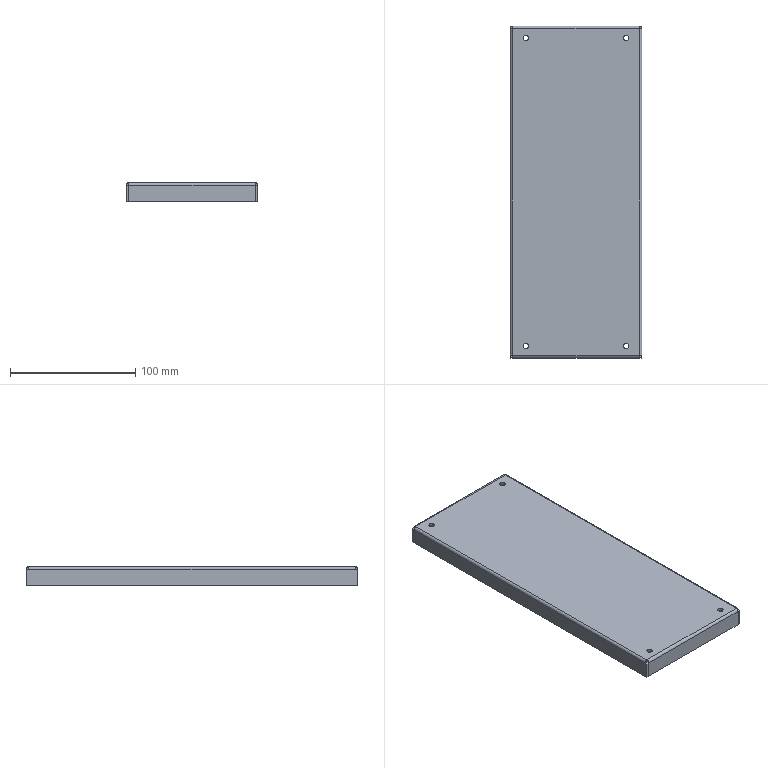Part | SolidWorks | features BaseBody 1 | 1 solid | 46 faces | box 105 x 265 x 15 mm | volume 73841 mm3 | plane 30 | cylinder 16 | commonest cylinder face diameters 4.2 x12 0.2 x4
STEP:
#1=CARTESIAN_POINT('',(37.9,-123.,-2.));
#2=VERTEX_POINT('',#1);
#3=CARTESIAN_POINT('',(42.1,-123.,-2.));
#4=VERTEX_POINT('',#3);
#5=CARTESIAN_POINT('',(40.,-123.,-2.));
#6=DIRECTION('',(0.,0.,1.));
#7=DIRECTION('',(1.,0.,0.));
#8=AXIS2_PLACEMENT_3D('',#5,#6,#7);
#9=CIRCLE('',#8,2.1);
#10=EDGE_CURVE('',#2,#4,#9,.T.);
#11=ORIENTED_EDGE('',*,*,#10,.F.);
#12=CARTESIAN_POINT('',(37.9,-123.,0.));
#13=VERTEX_POINT('',#12);
#14=CARTESIAN_POINT('',(37.9,-123.,0.));
#15=DIRECTION('',(0.,0.,1.));
#16=VECTOR('',#15,1000.);
#17=LINE('',#14,#16);
#18=EDGE_CURVE('',#2,#13,#17,.T.);
#19=ORIENTED_EDGE('',*,*,#18,.T.);
#20=CARTESIAN_POINT('',(42.1,-123.,0.));
#21=VERTEX_POINT('',#20);
#22=CARTESIAN_POINT('',(40.,-123.,0.));
#23=DIRECTION('',(0.,0.,-1.));
#24=DIRECTION('',(1.,0.,0.));
#25=AXIS2_PLACEMENT_3D('',#22,#23,#24);
#26=CIRCLE('',#25,2.1);
#27=EDGE_CURVE('',#21,#13,#26,.T.);
#28=ORIENTED_EDGE('',*,*,#27,.F.);
#29=CARTESIAN_POINT('',(42.1,-123.,0.));
#30=DIRECTION('',(0.,0.,1.));
#31=VECTOR('',#30,1000.);
#32=LINE('',#29,#31);
#33=EDGE_CURVE('',#4,#21,#32,.T.);
#34=ORIENTED_EDGE('',*,*,#33,.F.);
#35=EDGE_LOOP('',(#11,#19,#28,#34));
#36=FACE_OUTER_BOUND('',#35,.T.);
#37=CARTESIAN_POINT('',(40.,-123.,0.));
#38=DIRECTION('',(0.,0.,1.));
#39=DIRECTION('',(1.,0.,0.));
#40=AXIS2_PLACEMENT_3D('',#37,#38,#39);
#41=CYLINDRICAL_SURFACE('',#40,2.1);
#42=ADVANCED_FACE('',(#36),#41,.F.);
#43=CARTESIAN_POINT('',(-42.1,-123.,-2.));
#44=VERTEX_POINT('',#43);
#45=CARTESIAN_POINT('',(-37.9,-123.,-2.));
#46=VERTEX_POINT('',#45);
#47=CARTESIAN_POINT('',(-40.,-123.,-2.));
#48=DIRECTION('',(0.,0.,1.));
#49=DIRECTION('',(1.,0.,0.));
#50=AXIS2_PLACEMENT_3D('',#47,#48,#49);
#51=CIRCLE('',#50,2.1);
#52=EDGE_CURVE('',#44,#46,#51,.T.);
#53=ORIENTED_EDGE('',*,*,#52,.F.);
#54=CARTESIAN_POINT('',(-42.1,-123.,0.));
#55=VERTEX_POINT('',#54);
#56=CARTESIAN_POINT('',(-42.1,-123.,0.));
#57=DIRECTION('',(0.,0.,1.));
#58=VECTOR('',#57,1000.);
#59=LINE('',#56,#58);
#60=EDGE_CURVE('',#44,#55,#59,.T.);
#61=ORIENTED_EDGE('',*,*,#60,.T.);
#62=CARTESIAN_POINT('',(-37.9,-123.,0.));
#63=VERTEX_POINT('',#62);
#64=CARTESIAN_POINT('',(-40.,-123.,0.));
#65=DIRECTION('',(0.,0.,-1.));
#66=DIRECTION('',(1.,0.,0.));
#67=AXIS2_PLACEMENT_3D('',#64,#65,#66);
#68=CIRCLE('',#67,2.1);
#69=EDGE_CURVE('',#63,#55,#68,.T.);
#70=ORIENTED_EDGE('',*,*,#69,.F.);
#71=CARTESIAN_POINT('',(-37.9,-123.,0.));
#72=DIRECTION('',(0.,0.,1.));
#73=VECTOR('',#72,1000.);
#74=LINE('',#71,#73);
#75=EDGE_CURVE('',#46,#63,#74,.T.);
#76=ORIENTED_EDGE('',*,*,#75,.F.);
#77=EDGE_LOOP('',(#53,#61,#70,#76));
#78=FACE_OUTER_BOUND('',#77,.T.);
#79=CARTESIAN_POINT('',(-40.,-123.,0.));
#80=DIRECTION('',(0.,0.,1.));
#81=DIRECTION('',(1.,0.,0.));
#82=AXIS2_PLACEMENT_3D('',#79,#80,#81);
#83=CYLINDRICAL_SURFACE('',#82,2.1);
#84=ADVANCED_FACE('',(#78),#83,.F.);
#85=CARTESIAN_POINT('',(-42.1,123.,-2.));
#86=VERTEX_POINT('',#85);
#87=CARTESIAN_POINT('',(-37.9,123.,-2.));
#88=VERTEX_POINT('',#87);
#89=CARTESIAN_POINT('',(-40.,123.,-2.));
#90=DIRECTION('',(0.,0.,1.));
#91=DIRECTION('',(1.,0.,0.));
#92=AXIS2_PLACEMENT_3D('',#89,#90,#91);
#93=CIRCLE('',#92,2.1);
#94=EDGE_CURVE('',#86,#88,#93,.T.);
#95=ORIENTED_EDGE('',*,*,#94,.F.);
#96=CARTESIAN_POINT('',(-42.1,123.,0.));
#97=VERTEX_POINT('',#96);
#98=CARTESIAN_POINT('',(-42.1,123.,0.));
#99=DIRECTION('',(0.,0.,1.));
#100=VECTOR('',#99,1000.);
#101=LINE('',#98,#100);
#102=EDGE_CURVE('',#86,#97,#101,.T.);
#103=ORIENTED_EDGE('',*,*,#102,.T.);
#104=CARTESIAN_POINT('',(-37.9,123.,0.));
#105=VERTEX_POINT('',#104);
#106=CARTESIAN_POINT('',(-40.,123.,0.));
#107=DIRECTION('',(0.,0.,-1.));
#108=DIRECTION('',(1.,0.,0.));
#109=AXIS2_PLACEMENT_3D('',#106,#107,#108);
#110=CIRCLE('',#109,2.1);
#111=EDGE_CURVE('',#105,#97,#110,.T.);
#112=ORIENTED_EDGE('',*,*,#111,.F.);
#113=CARTESIAN_POINT('',(-37.9,123.,0.));
#114=DIRECTION('',(0.,0.,1.));
#115=VECTOR('',#114,1000.);
#116=LINE('',#113,#115);
#117=EDGE_CURVE('',#88,#105,#116,.T.);
#118=ORIENTED_EDGE('',*,*,#117,.F.);
#119=EDGE_LOOP('',(#95,#103,#112,#118));
#120=FACE_OUTER_BOUND('',#119,.T.);
#121=CARTESIAN_POINT('',(-40.,123.,0.));
#122=DIRECTION('',(0.,0.,1.));
#123=DIRECTION('',(1.,0.,0.));
#124=AXIS2_PLACEMENT_3D('',#121,#122,#123);
#125=CYLINDRICAL_SURFACE('',#124,2.1);
#126=ADVANCED_FACE('',(#120),#125,.F.);
#127=CARTESIAN_POINT('',(37.9,123.,-2.));
#128=VERTEX_POINT('',#127);
#129=CARTESIAN_POINT('',(42.1,123.,-2.));
#130=VERTEX_POINT('',#129);
#131=CARTESIAN_POINT('',(40.,123.,-2.));
#132=DIRECTION('',(0.,0.,1.));
#133=DIRECTION('',(1.,0.,0.));
#134=AXIS2_PLACEMENT_3D('',#131,#132,#133);
#135=CIRCLE('',#134,2.1);
#136=EDGE_CURVE('',#128,#130,#135,.T.);
#137=ORIENTED_EDGE('',*,*,#136,.F.);
#138=CARTESIAN_POINT('',(37.9,123.,0.));
#139=VERTEX_POINT('',#138);
#140=CARTESIAN_POINT('',(37.9,123.,0.));
#141=DIRECTION('',(0.,0.,1.));
#142=VECTOR('',#141,1000.);
#143=LINE('',#140,#142);
#144=EDGE_CURVE('',#128,#139,#143,.T.);
#145=ORIENTED_EDGE('',*,*,#144,.T.);
#146=CARTESIAN_POINT('',(42.1,123.,0.));
#147=VERTEX_POINT('',#146);
#148=CARTESIAN_POINT('',(40.,123.,0.));
#149=DIRECTION('',(0.,0.,-1.));
#150=DIRECTION('',(1.,0.,0.));
#151=AXIS2_PLACEMENT_3D('',#148,#149,#150);
#152=CIRCLE('',#151,2.1);
#153=EDGE_CURVE('',#147,#139,#152,.T.);
#154=ORIENTED_EDGE('',*,*,#153,.F.);
#155=CARTESIAN_POINT('',(42.1,123.,0.));
#156=DIRECTION('',(0.,0.,1.));
#157=VECTOR('',#156,1000.);
#158=LINE('',#155,#157);
#159=EDGE_CURVE('',#130,#147,#158,.T.);
#160=ORIENTED_EDGE('',*,*,#159,.F.);
#161=EDGE_LOOP('',(#137,#145,#154,#160));
#162=FACE_OUTER_BOUND('',#161,.T.);
#163=CARTESIAN_POINT('',(40.,123.,0.));
#164=DIRECTION('',(0.,0.,1.));
#165=DIRECTION('',(1.,0.,0.));
#166=AXIS2_PLACEMENT_3D('',#163,#164,#165);
#167=CYLINDRICAL_SURFACE('',#166,2.1);
#168=ADVANCED_FACE('',(#162),#167,.F.);
#169=ORIENTED_EDGE('',*,*,#27,.T.);
#170=CARTESIAN_POINT('',(40.,-123.,0.));
#171=DIRECTION('',(0.,0.,-1.));
#172=DIRECTION('',(1.,0.,0.));
#173=AXIS2_PLACEMENT_3D('',#170,#171,#172);
#174=CIRCLE('',#173,2.1);
#175=EDGE_CURVE('',#13,#21,#174,.T.);
#176=ORIENTED_EDGE('',*,*,#175,.T.);
#177=EDGE_LOOP('',(#169,#176));
#178=FACE_BOUND('',#177,.T.);
#179=ORIENTED_EDGE('',*,*,#69,.T.);
#180=CARTESIAN_POINT('',(-40.,-123.,0.));
#181=DIRECTION('',(0.,0.,-1.));
#182=DIRECTION('',(1.,0.,0.));
#183=AXIS2_PLACEMENT_3D('',#180,#181,#182);
#184=CIRCLE('',#183,2.1);
#185=EDGE_CURVE('',#55,#63,#184,.T.);
#186=ORIENTED_EDGE('',*,*,#185,.T.);
#187=EDGE_LOOP('',(#179,#186));
#188=FACE_BOUND('',#187,.T.);
#189=CARTESIAN_POINT('',(50.4,-130.4,0.));
#190=VERTEX_POINT('',#189);
#191=CARTESIAN_POINT('',(50.4,130.4,0.));
#192=VERTEX_POINT('',#191);
#193=CARTESIAN_POINT('',(50.4,0.,0.));
#194=DIRECTION('',(0.,1.,0.));
#195=VECTOR('',#194,1000.);
#196=LINE('',#193,#195);
#197=EDGE_CURVE('',#190,#192,#196,.T.);
#198=ORIENTED_EDGE('',*,*,#197,.T.);
#199=CARTESIAN_POINT('',(-50.4,130.4,0.));
#200=VERTEX_POINT('',#199);
#201=CARTESIAN_POINT('',(0.,130.4,0.));
#202=DIRECTION('',(-1.,0.,0.));
#203=VECTOR('',#202,1000.);
#204=LINE('',#201,#203);
#205=EDGE_CURVE('',#192,#200,#204,.T.);
#206=ORIENTED_EDGE('',*,*,#205,.T.);
#207=CARTESIAN_POINT('',(-50.4,-130.4,0.));
#208=VERTEX_POINT('',#207);
#209=CARTESIAN_POINT('',(-50.4,0.,0.));
#210=DIRECTION('',(0.,-1.,0.));
#211=VECTOR('',#210,1000.);
#212=LINE('',#209,#211);
#213=EDGE_CURVE('',#200,#208,#212,.T.);
#214=ORIENTED_EDGE('',*,*,#213,.T.);
#215=CARTESIAN_POINT('',(0.,-130.4,0.));
#216=DIRECTION('',(1.,0.,0.));
#217=VECTOR('',#216,1000.);
#218=LINE('',#215,#217);
#219=EDGE_CURVE('',#208,#190,#218,.T.);
#220=ORIENTED_EDGE('',*,*,#219,.T.);
#221=EDGE_LOOP('',(#198,#206,#214,#220));
#222=FACE_OUTER_BOUND('',#221,.T.);
#223=ORIENTED_EDGE('',*,*,#111,.T.);
#224=CARTESIAN_POINT('',(-40.,123.,0.));
#225=DIRECTION('',(0.,0.,-1.));
#226=DIRECTION('',(1.,0.,0.));
#227=AXIS2_PLACEMENT_3D('',#224,#225,#226);
#228=CIRCLE('',#227,2.1);
#229=EDGE_CURVE('',#97,#105,#228,.T.);
#230=ORIENTED_EDGE('',*,*,#229,.T.);
#231=EDGE_LOOP('',(#223,#230));
#232=FACE_BOUND('',#231,.T.);
#233=ORIENTED_EDGE('',*,*,#153,.T.);
#234=CARTESIAN_POINT('',(40.,123.,0.));
#235=DIRECTION('',(0.,0.,-1.));
#236=DIRECTION('',(1.,0.,0.));
#237=AXIS2_PLACEMENT_3D('',#234,#235,#236);
#238=CIRCLE('',#237,2.1);
#239=EDGE_CURVE('',#139,#147,#238,.T.);
#240=ORIENTED_EDGE('',*,*,#239,.T.);
#241=EDGE_LOOP('',(#233,#240));
#242=FACE_BOUND('',#241,.T.);
#243=CARTESIAN_POINT('',(0.,0.,0.));
#244=DIRECTION('',(0.,0.,1.));
#245=DIRECTION('',(1.,0.,0.));
#246=AXIS2_PLACEMENT_3D('',#243,#244,#245);
#247=PLANE('',#246);
#248=ADVANCED_FACE('',(#178,#188,#222,#232,#242),#247,.T.);
#249=ORIENTED_EDGE('',*,*,#18,.F.);
#250=CARTESIAN_POINT('',(40.,-123.,-2.));
#251=DIRECTION('',(0.,0.,1.));
#252=DIRECTION('',(1.,0.,0.));
#253=AXIS2_PLACEMENT_3D('',#250,#251,#252);
#254=CIRCLE('',#253,2.1);
#255=EDGE_CURVE('',#4,#2,#254,.T.);
#256=ORIENTED_EDGE('',*,*,#255,.F.);
#257=ORIENTED_EDGE('',*,*,#33,.T.);
#258=ORIENTED_EDGE('',*,*,#175,.F.);
#259=EDGE_LOOP('',(#249,#256,#257,#258));
#260=FACE_OUTER_BOUND('',#259,.T.);
#261=CARTESIAN_POINT('',(40.,-123.,0.));
#262=DIRECTION('',(0.,0.,1.));
#263=DIRECTION('',(1.,0.,0.));
#264=AXIS2_PLACEMENT_3D('',#261,#262,#263);
#265=CYLINDRICAL_SURFACE('',#264,2.1);
#266=ADVANCED_FACE('',(#260),#265,.F.);
#267=ORIENTED_EDGE('',*,*,#60,.F.);
#268=CARTESIAN_POINT('',(-40.,-123.,-2.));
#269=DIRECTION('',(0.,0.,1.));
#270=DIRECTION('',(1.,0.,0.));
#271=AXIS2_PLACEMENT_3D('',#268,#269,#270);
#272=CIRCLE('',#271,2.1);
#273=EDGE_CURVE('',#46,#44,#272,.T.);
#274=ORIENTED_EDGE('',*,*,#273,.F.);
#275=ORIENTED_EDGE('',*,*,#75,.T.);
#276=ORIENTED_EDGE('',*,*,#185,.F.);
#277=EDGE_LOOP('',(#267,#274,#275,#276));
#278=FACE_OUTER_BOUND('',#277,.T.);
#279=CARTESIAN_POINT('',(-40.,-123.,0.));
#280=DIRECTION('',(0.,0.,1.));
#281=DIRECTION('',(1.,0.,0.));
#282=AXIS2_PLACEMENT_3D('',#279,#280,#281);
#283=CYLINDRICAL_SURFACE('',#282,2.1);
#284=ADVANCED_FACE('',(#278),#283,.F.);
#285=CARTESIAN_POINT('',(50.4,132.5,-2.1));
#286=VERTEX_POINT('',#285);
#287=CARTESIAN_POINT('',(-50.4,132.5,-2.1));
#288=VERTEX_POINT('',#287);
#289=CARTESIAN_POINT('',(50.4,132.5,-2.1));
#290=DIRECTION('',(-1.,0.,0.));
#291=VECTOR('',#290,1000.);
#292=LINE('',#289,#291);
#293=EDGE_CURVE('',#286,#288,#292,.T.);
#294=ORIENTED_EDGE('',*,*,#293,.T.);
#295=CARTESIAN_POINT('',(-50.4,130.4,-2.1));
#296=DIRECTION('',(1.,0.,0.));
#297=DIRECTION('',(0.,0.,-1.));
#298=AXIS2_PLACEMENT_3D('',#295,#296,#297);
#299=CIRCLE('',#298,2.1);
#300=EDGE_CURVE('',#288,#200,#299,.T.);
#301=ORIENTED_EDGE('',*,*,#300,.T.);
#302=ORIENTED_EDGE('',*,*,#205,.F.);
#303=CARTESIAN_POINT('',(50.4,130.4,-2.1));
#304=DIRECTION('',(-1.,0.,0.));
#305=DIRECTION('',(0.,0.,-1.));
#306=AXIS2_PLACEMENT_3D('',#303,#304,#305);
#307=CIRCLE('',#306,2.1);
#308=EDGE_CURVE('',#192,#286,#307,.T.);
#309=ORIENTED_EDGE('',*,*,#308,.T.);
#310=EDGE_LOOP('',(#294,#301,#302,#309));
#311=FACE_OUTER_BOUND('',#310,.T.);
#312=CARTESIAN_POINT('',(50.4,130.4,-2.1));
#313=DIRECTION('',(1.,0.,0.));
#314=DIRECTION('',(0.,0.,-1.));
#315=AXIS2_PLACEMENT_3D('',#312,#313,#314);
#316=CYLINDRICAL_SURFACE('',#315,2.1);
#317=ADVANCED_FACE('',(#311),#316,.T.);
#318=CARTESIAN_POINT('',(52.5,-130.4,-2.1));
#319=VERTEX_POINT('',#318);
#320=CARTESIAN_POINT('',(52.5,130.4,-2.1));
#321=VERTEX_POINT('',#320);
#322=CARTESIAN_POINT('',(52.5,-132.5,-2.1));
#323=DIRECTION('',(0.,1.,0.));
#324=VECTOR('',#323,1000.);
#325=LINE('',#322,#324);
#326=EDGE_CURVE('',#319,#321,#325,.T.);
#327=ORIENTED_EDGE('',*,*,#326,.T.);
#328=CARTESIAN_POINT('',(50.4,130.4,-2.1));
#329=DIRECTION('',(0.,-1.,0.));
#330=DIRECTION('',(0.,0.,-1.));
#331=AXIS2_PLACEMENT_3D('',#328,#329,#330);
#332=CIRCLE('',#331,2.1);
#333=EDGE_CURVE('',#321,#192,#332,.T.);
#334=ORIENTED_EDGE('',*,*,#333,.T.);
#335=ORIENTED_EDGE('',*,*,#197,.F.);
#336=CARTESIAN_POINT('',(50.4,-130.4,-2.1));
#337=DIRECTION('',(0.,1.,0.));
#338=DIRECTION('',(0.,0.,-1.));
#339=AXIS2_PLACEMENT_3D('',#336,#337,#338);
#340=CIRCLE('',#339,2.1);
#341=EDGE_CURVE('',#190,#319,#340,.T.);
#342=ORIENTED_EDGE('',*,*,#341,.T.);
#343=EDGE_LOOP('',(#327,#334,#335,#342));
#344=FACE_OUTER_BOUND('',#343,.T.);
#345=CARTESIAN_POINT('',(50.4,-132.5,-2.1));
#346=DIRECTION('',(0.,-1.,0.));
#347=DIRECTION('',(0.,0.,-1.));
#348=AXIS2_PLACEMENT_3D('',#345,#346,#347);
#349=CYLINDRICAL_SURFACE('',#348,2.1);
#350=ADVANCED_FACE('',(#344),#349,.T.);
#351=CARTESIAN_POINT('',(-50.4,-132.5,-2.1));
#352=VERTEX_POINT('',#351);
#353=CARTESIAN_POINT('',(50.4,-132.5,-2.1));
#354=VERTEX_POINT('',#353);
#355=CARTESIAN_POINT('',(-50.4,-132.5,-2.1));
#356=DIRECTION('',(1.,0.,0.));
#357=VECTOR('',#356,1000.);
#358=LINE('',#355,#357);
#359=EDGE_CURVE('',#352,#354,#358,.T.);
#360=ORIENTED_EDGE('',*,*,#359,.T.);
#361=CARTESIAN_POINT('',(50.4,-130.4,-2.1));
#362=DIRECTION('',(-1.,0.,0.));
#363=DIRECTION('',(0.,0.,1.));
#364=AXIS2_PLACEMENT_3D('',#361,#362,#363);
#365=CIRCLE('',#364,2.1);
#366=EDGE_CURVE('',#354,#190,#365,.T.);
#367=ORIENTED_EDGE('',*,*,#366,.T.);
#368=ORIENTED_EDGE('',*,*,#219,.F.);
#369=CARTESIAN_POINT('',(-50.4,-130.4,-2.1));
#370=DIRECTION('',(1.,0.,0.));
#371=DIRECTION('',(0.,0.,1.));
#372=AXIS2_PLACEMENT_3D('',#369,#370,#371);
#373=CIRCLE('',#372,2.1);
#374=EDGE_CURVE('',#208,#352,#373,.T.);
#375=ORIENTED_EDGE('',*,*,#374,.T.);
#376=EDGE_LOOP('',(#360,#367,#368,#375));
#377=FACE_OUTER_BOUND('',#376,.T.);
#378=CARTESIAN_POINT('',(-50.4,-130.4,-2.1));
#379=DIRECTION('',(-1.,0.,0.));
#380=DIRECTION('',(0.,0.,1.));
#381=AXIS2_PLACEMENT_3D('',#378,#379,#380);
#382=CYLINDRICAL_SURFACE('',#381,2.1);
#383=ADVANCED_FACE('',(#377),#382,.T.);
#384=ORIENTED_EDGE('',*,*,#213,.F.);
#385=CARTESIAN_POINT('',(-52.5,130.4,-2.1));
#386=VERTEX_POINT('',#385);
#387=CARTESIAN_POINT('',(-50.4,130.4,-2.1));
#388=DIRECTION('',(0.,-1.,0.));
#389=DIRECTION('',(0.,0.,1.));
#390=AXIS2_PLACEMENT_3D('',#387,#388,#389);
#391=CIRCLE('',#390,2.1);
#392=EDGE_CURVE('',#200,#386,#391,.T.);
#393=ORIENTED_EDGE('',*,*,#392,.T.);
#394=CARTESIAN_POINT('',(-52.5,-130.4,-2.1));
#395=VERTEX_POINT('',#394);
#396=CARTESIAN_POINT('',(-52.5,132.5,-2.1));
#397=DIRECTION('',(0.,-1.,0.));
#398=VECTOR('',#397,1000.);
#399=LINE('',#396,#398);
#400=EDGE_CURVE('',#386,#395,#399,.T.);
#401=ORIENTED_EDGE('',*,*,#400,.T.);
#402=CARTESIAN_POINT('',(-50.4,-130.4,-2.1));
#403=DIRECTION('',(0.,1.,0.));
#404=DIRECTION('',(0.,0.,1.));
#405=AXIS2_PLACEMENT_3D('',#402,#403,#404);
#406=CIRCLE('',#405,2.1);
#407=EDGE_CURVE('',#395,#208,#406,.T.);
#408=ORIENTED_EDGE('',*,*,#407,.T.);
#409=EDGE_LOOP('',(#384,#393,#401,#408));
#410=FACE_OUTER_BOUND('',#409,.T.);
#411=CARTESIAN_POINT('',(-50.4,132.5,-2.1));
#412=DIRECTION('',(0.,1.,0.));
#413=DIRECTION('',(0.,0.,1.));
#414=AXIS2_PLACEMENT_3D('',#411,#412,#413);
#415=CYLINDRICAL_SURFACE('',#414,2.1);
#416=ADVANCED_FACE('',(#410),#415,.T.);
#417=ORIENTED_EDGE('',*,*,#102,.F.);
#418=CARTESIAN_POINT('',(-40.,123.,-2.));
#419=DIRECTION('',(0.,0.,1.));
#420=DIRECTION('',(1.,0.,0.));
#421=AXIS2_PLACEMENT_3D('',#418,#419,#420);
#422=CIRCLE('',#421,2.1);
#423=EDGE_CURVE('',#88,#86,#422,.T.);
#424=ORIENTED_EDGE('',*,*,#423,.F.);
#425=ORIENTED_EDGE('',*,*,#117,.T.);
#426=ORIENTED_EDGE('',*,*,#229,.F.);
#427=EDGE_LOOP('',(#417,#424,#425,#426));
#428=FACE_OUTER_BOUND('',#427,.T.);
#429=CARTESIAN_POINT('',(-40.,123.,0.));
#430=DIRECTION('',(0.,0.,1.));
#431=DIRECTION('',(1.,0.,0.));
#432=AXIS2_PLACEMENT_3D('',#429,#430,#431);
#433=CYLINDRICAL_SURFACE('',#432,2.1);
#434=ADVANCED_FACE('',(#428),#433,.F.);
#435=ORIENTED_EDGE('',*,*,#144,.F.);
#436=CARTESIAN_POINT('',(40.,123.,-2.));
#437=DIRECTION('',(0.,0.,1.));
#438=DIRECTION('',(1.,0.,0.));
#439=AXIS2_PLACEMENT_3D('',#436,#437,#438);
#440=CIRCLE('',#439,2.1);
#441=EDGE_CURVE('',#130,#128,#440,.T.);
#442=ORIENTED_EDGE('',*,*,#441,.F.);
#443=ORIENTED_EDGE('',*,*,#159,.T.);
#444=ORIENTED_EDGE('',*,*,#239,.F.);
#445=EDGE_LOOP('',(#435,#442,#443,#444));
#446=FACE_OUTER_BOUND('',#445,.T.);
#447=CARTESIAN_POINT('',(40.,123.,0.));
#448=DIRECTION('',(0.,0.,1.));
#449=DIRECTION('',(1.,0.,0.));
#450=AXIS2_PLACEMENT_3D('',#447,#448,#449);
#451=CYLINDRICAL_SURFACE('',#450,2.1);
#452=ADVANCED_FACE('',(#446),#451,.F.);
#453=ORIENTED_EDGE('',*,*,#255,.T.);
#454=ORIENTED_EDGE('',*,*,#10,.T.);
#455=EDGE_LOOP('',(#453,#454));
#456=FACE_BOUND('',#455,.T.);
#457=ORIENTED_EDGE('',*,*,#273,.T.);
#458=ORIENTED_EDGE('',*,*,#52,.T.);
#459=EDGE_LOOP('',(#457,#458));
#460=FACE_BOUND('',#459,.T.);
#461=CARTESIAN_POINT('',(-50.4,130.4,-2.));
#462=VERTEX_POINT('',#461);
#463=CARTESIAN_POINT('',(-50.4,-130.4,-2.));
#464=VERTEX_POINT('',#463);
#465=CARTESIAN_POINT('',(-50.4,0.,-2.));
#466=DIRECTION('',(0.,-1.,0.));
#467=VECTOR('',#466,1000.);
#468=LINE('',#465,#467);
#469=EDGE_CURVE('',#462,#464,#468,.T.);
#470=ORIENTED_EDGE('',*,*,#469,.F.);
#471=CARTESIAN_POINT('',(50.4,130.4,-2.));
#472=VERTEX_POINT('',#471);
#473=CARTESIAN_POINT('',(0.,130.4,-2.));
#474=DIRECTION('',(-1.,0.,0.));
#475=VECTOR('',#474,1000.);
#476=LINE('',#473,#475);
#477=EDGE_CURVE('',#472,#462,#476,.T.);
#478=ORIENTED_EDGE('',*,*,#477,.F.);
#479=CARTESIAN_POINT('',(50.4,-130.4,-2.));
#480=VERTEX_POINT('',#479);
#481=CARTESIAN_POINT('',(50.4,0.,-2.));
#482=DIRECTION('',(0.,1.,0.));
#483=VECTOR('',#482,1000.);
#484=LINE('',#481,#483);
#485=EDGE_CURVE('',#480,#472,#484,.T.);
#486=ORIENTED_EDGE('',*,*,#485,.F.);
#487=CARTESIAN_POINT('',(0.,-130.4,-2.));
#488=DIRECTION('',(1.,0.,0.));
#489=VECTOR('',#488,1000.);
#490=LINE('',#487,#489);
#491=EDGE_CURVE('',#464,#480,#490,.T.);
#492=ORIENTED_EDGE('',*,*,#491,.F.);
#493=EDGE_LOOP('',(#470,#478,#486,#492));
#494=FACE_OUTER_BOUND('',#493,.T.);
#495=ORIENTED_EDGE('',*,*,#423,.T.);
#496=ORIENTED_EDGE('',*,*,#94,.T.);
#497=EDGE_LOOP('',(#495,#496));
#498=FACE_BOUND('',#497,.T.);
#499=ORIENTED_EDGE('',*,*,#441,.T.);
#500=ORIENTED_EDGE('',*,*,#136,.T.);
#501=EDGE_LOOP('',(#499,#500));
#502=FACE_BOUND('',#501,.T.);
#503=CARTESIAN_POINT('',(0.,0.,-2.));
#504=DIRECTION('',(0.,0.,1.));
#505=DIRECTION('',(1.,0.,0.));
#506=AXIS2_PLACEMENT_3D('',#503,#504,#505);
#507=PLANE('',#506);
#508=ADVANCED_FACE('',(#456,#460,#494,#498,#502),#507,.F.);
#509=CARTESIAN_POINT('',(-50.4,130.4,-2.1));
#510=DIRECTION('',(0.,0.,1.));
#511=VECTOR('',#510,1000.);
#512=LINE('',#509,#511);
#513=EDGE_CURVE('',#462,#200,#512,.T.);
#514=ORIENTED_EDGE('',*,*,#513,.T.);
#515=ORIENTED_EDGE('',*,*,#300,.F.);
#516=CARTESIAN_POINT('',(-50.4,132.5,-15.));
#517=VERTEX_POINT('',#516);
#518=CARTESIAN_POINT('',(-50.4,132.5,0.));
#519=DIRECTION('',(0.,0.,1.));
#520=VECTOR('',#519,1000.);
#521=LINE('',#518,#520);
#522=EDGE_CURVE('',#517,#288,#521,.T.);
#523=ORIENTED_EDGE('',*,*,#522,.F.);
#524=CARTESIAN_POINT('',(-50.4,130.5,-15.));
#525=VERTEX_POINT('',#524);
#526=CARTESIAN_POINT('',(-50.4,132.5,-15.));
#527=DIRECTION('',(0.,-1.,0.));
#528=VECTOR('',#527,1000.);
#529=LINE('',#526,#528);
#530=EDGE_CURVE('',#517,#525,#529,.T.);
#531=ORIENTED_EDGE('',*,*,#530,.T.);
#532=CARTESIAN_POINT('',(-50.4,130.5,-2.1));
#533=VERTEX_POINT('',#532);
#534=CARTESIAN_POINT('',(-50.4,130.5,-15.));
#535=DIRECTION('',(0.,0.,1.));
#536=VECTOR('',#535,1000.);
#537=LINE('',#534,#536);
#538=EDGE_CURVE('',#525,#533,#537,.T.);
#539=ORIENTED_EDGE('',*,*,#538,.T.);
#540=CARTESIAN_POINT('',(-50.4,130.4,-2.1));
#541=DIRECTION('',(1.,0.,0.));
#542=DIRECTION('',(0.,0.,-1.));
#543=AXIS2_PLACEMENT_3D('',#540,#541,#542);
#544=CIRCLE('',#543,0.1);
#545=EDGE_CURVE('',#533,#462,#544,.T.);
#546=ORIENTED_EDGE('',*,*,#545,.T.);
#547=EDGE_LOOP('',(#514,#515,#523,#531,#539,#546));
#548=FACE_OUTER_BOUND('',#547,.T.);
#549=CARTESIAN_POINT('',(-50.4,130.4,-2.1));
#550=DIRECTION('',(-1.,0.,0.));
#551=DIRECTION('',(0.,0.,1.));
#552=AXIS2_PLACEMENT_3D('',#549,#550,#551);
#553=PLANE('',#552);
#554=ADVANCED_FACE('',(#548),#553,.T.);
#555=CARTESIAN_POINT('',(50.4,132.5,-15.));
#556=VERTEX_POINT('',#555);
#557=CARTESIAN_POINT('',(50.4,132.5,0.));
#558=DIRECTION('',(0.,0.,-1.));
#559=VECTOR('',#558,1000.);
#560=LINE('',#557,#559);
#561=EDGE_CURVE('',#286,#556,#560,.T.);
#562=ORIENTED_EDGE('',*,*,#561,.T.);
#563=CARTESIAN_POINT('',(0.,132.5,-15.));
#564=DIRECTION('',(-1.,0.,0.));
#565=VECTOR('',#564,1000.);
#566=LINE('',#563,#565);
#567=EDGE_CURVE('',#556,#517,#566,.T.);
#568=ORIENTED_EDGE('',*,*,#567,.T.);
#569=ORIENTED_EDGE('',*,*,#522,.T.);
#570=ORIENTED_EDGE('',*,*,#293,.F.);
#571=EDGE_LOOP('',(#562,#568,#569,#570));
#572=FACE_OUTER_BOUND('',#571,.T.);
#573=CARTESIAN_POINT('',(0.,132.5,0.));
#574=DIRECTION('',(0.,1.,0.));
#575=DIRECTION('',(0.,0.,1.));
#576=AXIS2_PLACEMENT_3D('',#573,#574,#575);
#577=PLANE('',#576);
#578=ADVANCED_FACE('',(#572),#577,.T.);
#579=CARTESIAN_POINT('',(50.4,130.5,-2.1));
#580=VERTEX_POINT('',#579);
#581=CARTESIAN_POINT('',(50.4,130.4,-2.1));
#582=DIRECTION('',(1.,0.,0.));
#583=DIRECTION('',(0.,0.,-1.));
#584=AXIS2_PLACEMENT_3D('',#581,#582,#583);
#585=CIRCLE('',#584,0.1);
#586=EDGE_CURVE('',#580,#472,#585,.T.);
#587=ORIENTED_EDGE('',*,*,#586,.F.);
#588=CARTESIAN_POINT('',(50.4,130.5,-15.));
#589=VERTEX_POINT('',#588);
#590=CARTESIAN_POINT('',(50.4,130.5,-2.));
#591=DIRECTION('',(0.,0.,-1.));
#592=VECTOR('',#591,1000.);
#593=LINE('',#590,#592);
#594=EDGE_CURVE('',#580,#589,#593,.T.);
#595=ORIENTED_EDGE('',*,*,#594,.T.);
#596=CARTESIAN_POINT('',(50.4,132.5,-15.));
#597=DIRECTION('',(0.,-1.,0.));
#598=VECTOR('',#597,1000.);
#599=LINE('',#596,#598);
#600=EDGE_CURVE('',#556,#589,#599,.T.);
#601=ORIENTED_EDGE('',*,*,#600,.F.);
#602=ORIENTED_EDGE('',*,*,#561,.F.);
#603=ORIENTED_EDGE('',*,*,#308,.F.);
#604=CARTESIAN_POINT('',(50.4,130.4,-2.1));
#605=DIRECTION('',(0.,0.,1.));
#606=VECTOR('',#605,1000.);
#607=LINE('',#604,#606);
#608=EDGE_CURVE('',#472,#192,#607,.T.);
#609=ORIENTED_EDGE('',*,*,#608,.F.);
#610=EDGE_LOOP('',(#587,#595,#601,#602,#603,#609));
#611=FACE_OUTER_BOUND('',#610,.T.);
#612=CARTESIAN_POINT('',(50.4,130.4,-2.1));
#613=DIRECTION('',(-1.,0.,0.));
#614=DIRECTION('',(0.,0.,1.));
#615=AXIS2_PLACEMENT_3D('',#612,#613,#614);
#616=PLANE('',#615);
#617=ADVANCED_FACE('',(#611),#616,.F.);
#618=CARTESIAN_POINT('',(50.5,130.4,-2.1));
#619=VERTEX_POINT('',#618);
#620=CARTESIAN_POINT('',(50.4,130.4,-2.1));
#621=DIRECTION('',(0.,-1.,0.));
#622=DIRECTION('',(0.,0.,-1.));
#623=AXIS2_PLACEMENT_3D('',#620,#621,#622);
#624=CIRCLE('',#623,0.1);
#625=EDGE_CURVE('',#619,#472,#624,.T.);
#626=ORIENTED_EDGE('',*,*,#625,.T.);
#627=ORIENTED_EDGE('',*,*,#608,.T.);
#628=ORIENTED_EDGE('',*,*,#333,.F.);
#629=CARTESIAN_POINT('',(50.4,130.4,-2.1));
#630=DIRECTION('',(-1.,0.,0.));
#631=VECTOR('',#630,1000.);
#632=LINE('',#629,#631);
#633=EDGE_CURVE('',#321,#619,#632,.T.);
#634=ORIENTED_EDGE('',*,*,#633,.T.);
#635=EDGE_LOOP('',(#626,#627,#628,#634));
#636=FACE_OUTER_BOUND('',#635,.T.);
#637=CARTESIAN_POINT('',(50.4,130.4,-2.1));
#638=DIRECTION('',(0.,1.,0.));
#639=DIRECTION('',(0.,0.,1.));
#640=AXIS2_PLACEMENT_3D('',#637,#638,#639);
#641=PLANE('',#640);
#642=ADVANCED_FACE('',(#636),#641,.T.);
#643=CARTESIAN_POINT('',(52.5,-132.5,-2.1));
#644=VERTEX_POINT('',#643);
#645=CARTESIAN_POINT('',(52.5,-132.5,-15.));
#646=VERTEX_POINT('',#645);
#647=CARTESIAN_POINT('',(52.5,-132.5,0.));
#648=DIRECTION('',(0.,0.,-1.));
#649=VECTOR('',#648,1000.);
#650=LINE('',#647,#649);
#651=EDGE_CURVE('',#644,#646,#650,.T.);
#652=ORIENTED_EDGE('',*,*,#651,.T.);
#653=CARTESIAN_POINT('',(52.5,132.5,-15.));
#654=VERTEX_POINT('',#653);
#655=CARTESIAN_POINT('',(52.5,0.,-15.));
#656=DIRECTION('',(0.,1.,0.));
#657=VECTOR('',#656,1000.);
#658=LINE('',#655,#657);
#659=EDGE_CURVE('',#646,#654,#658,.T.);
#660=ORIENTED_EDGE('',*,*,#659,.T.);
#661=CARTESIAN_POINT('',(52.5,132.5,-2.1));
#662=VERTEX_POINT('',#661);
#663=CARTESIAN_POINT('',(52.5,132.5,0.));
#664=DIRECTION('',(0.,0.,1.));
#665=VECTOR('',#664,1000.);
#666=LINE('',#663,#665);
#667=EDGE_CURVE('',#654,#662,#666,.T.);
#668=ORIENTED_EDGE('',*,*,#667,.T.);
#669=CARTESIAN_POINT('',(52.5,0.,-2.1));
#670=DIRECTION('',(0.,-1.,0.));
#671=VECTOR('',#670,1000.);
#672=LINE('',#669,#671);
#673=EDGE_CURVE('',#662,#321,#672,.T.);
#674=ORIENTED_EDGE('',*,*,#673,.T.);
#675=ORIENTED_EDGE('',*,*,#326,.F.);
#676=CARTESIAN_POINT('',(52.5,0.,-2.1));
#677=DIRECTION('',(0.,-1.,0.));
#678=VECTOR('',#677,1000.);
#679=LINE('',#676,#678);
#680=EDGE_CURVE('',#319,#644,#679,.T.);
#681=ORIENTED_EDGE('',*,*,#680,.T.);
#682=EDGE_LOOP('',(#652,#660,#668,#674,#675,#681));
#683=FACE_OUTER_BOUND('',#682,.T.);
#684=CARTESIAN_POINT('',(52.5,0.,0.));
#685=DIRECTION('',(1.,0.,0.));
#686=DIRECTION('',(0.,0.,-1.));
#687=AXIS2_PLACEMENT_3D('',#684,#685,#686);
#688=PLANE('',#687);
#689=ADVANCED_FACE('',(#683),#688,.T.);
#690=ORIENTED_EDGE('',*,*,#341,.F.);
#691=CARTESIAN_POINT('',(50.4,-130.4,-2.1));
#692=DIRECTION('',(0.,0.,-1.));
#693=VECTOR('',#692,1000.);
#694=LINE('',#691,#693);
#695=EDGE_CURVE('',#190,#480,#694,.T.);
#696=ORIENTED_EDGE('',*,*,#695,.T.);
#697=CARTESIAN_POINT('',(50.5,-130.4,-2.1));
#698=VERTEX_POINT('',#697);
#699=CARTESIAN_POINT('',(50.4,-130.4,-2.1));
#700=DIRECTION('',(0.,1.,0.));
#701=DIRECTION('',(0.,0.,-1.));
#702=AXIS2_PLACEMENT_3D('',#699,#700,#701);
#703=CIRCLE('',#702,0.1);
#704=EDGE_CURVE('',#480,#698,#703,.T.);
#705=ORIENTED_EDGE('',*,*,#704,.T.);
#706=CARTESIAN_POINT('',(50.4,-130.4,-2.1));
#707=DIRECTION('',(1.,0.,0.));
#708=VECTOR('',#707,1000.);
#709=LINE('',#706,#708);
#710=EDGE_CURVE('',#698,#319,#709,.T.);
#711=ORIENTED_EDGE('',*,*,#710,.T.);
#712=EDGE_LOOP('',(#690,#696,#705,#711));
#713=FACE_OUTER_BOUND('',#712,.T.);
#714=CARTESIAN_POINT('',(50.4,-130.4,-2.1));
#715=DIRECTION('',(0.,-1.,0.));
#716=DIRECTION('',(0.,0.,-1.));
#717=AXIS2_PLACEMENT_3D('',#714,#715,#716);
#718=PLANE('',#717);
#719=ADVANCED_FACE('',(#713),#718,.T.);
#720=ORIENTED_EDGE('',*,*,#695,.F.);
#721=ORIENTED_EDGE('',*,*,#366,.F.);
#722=CARTESIAN_POINT('',(50.4,-132.5,-15.));
#723=VERTEX_POINT('',#722);
#724=CARTESIAN_POINT('',(50.4,-132.5,0.));
#725=DIRECTION('',(0.,0.,-1.));
#726=VECTOR('',#725,1000.);
#727=LINE('',#724,#726);
#728=EDGE_CURVE('',#354,#723,#727,.T.);
#729=ORIENTED_EDGE('',*,*,#728,.T.);
#730=CARTESIAN_POINT('',(50.4,-130.5,-15.));
#731=VERTEX_POINT('',#730);
#732=CARTESIAN_POINT('',(50.4,-132.5,-15.));
#733=DIRECTION('',(0.,1.,0.));
#734=VECTOR('',#733,1000.);
#735=LINE('',#732,#734);
#736=EDGE_CURVE('',#723,#731,#735,.T.);
#737=ORIENTED_EDGE('',*,*,#736,.T.);
#738=CARTESIAN_POINT('',(50.4,-130.5,-2.1));
#739=VERTEX_POINT('',#738);
#740=CARTESIAN_POINT('',(50.4,-130.5,-2.));
#741=DIRECTION('',(0.,0.,1.));
#742=VECTOR('',#741,1000.);
#743=LINE('',#740,#742);
#744=EDGE_CURVE('',#731,#739,#743,.T.);
#745=ORIENTED_EDGE('',*,*,#744,.T.);
#746=CARTESIAN_POINT('',(50.4,-130.4,-2.1));
#747=DIRECTION('',(-1.,0.,0.));
#748=DIRECTION('',(0.,0.,1.));
#749=AXIS2_PLACEMENT_3D('',#746,#747,#748);
#750=CIRCLE('',#749,0.1);
#751=EDGE_CURVE('',#739,#480,#750,.T.);
#752=ORIENTED_EDGE('',*,*,#751,.T.);
#753=EDGE_LOOP('',(#720,#721,#729,#737,#745,#752));
#754=FACE_OUTER_BOUND('',#753,.T.);
#755=CARTESIAN_POINT('',(50.4,-130.4,-2.1));
#756=DIRECTION('',(1.,0.,0.));
#757=DIRECTION('',(0.,0.,-1.));
#758=AXIS2_PLACEMENT_3D('',#755,#756,#757);
#759=PLANE('',#758);
#760=ADVANCED_FACE('',(#754),#759,.T.);
#761=CARTESIAN_POINT('',(-50.4,-132.5,-15.));
#762=VERTEX_POINT('',#761);
#763=CARTESIAN_POINT('',(-50.4,-132.5,0.));
#764=DIRECTION('',(0.,0.,1.));
#765=VECTOR('',#764,1000.);
#766=LINE('',#763,#765);
#767=EDGE_CURVE('',#762,#352,#766,.T.);
#768=ORIENTED_EDGE('',*,*,#767,.F.);
#769=CARTESIAN_POINT('',(0.,-132.5,-15.));
#770=DIRECTION('',(-1.,0.,0.));
#771=VECTOR('',#770,1000.);
#772=LINE('',#769,#771);
#773=EDGE_CURVE('',#723,#762,#772,.T.);
#774=ORIENTED_EDGE('',*,*,#773,.F.);
#775=ORIENTED_EDGE('',*,*,#728,.F.);
#776=ORIENTED_EDGE('',*,*,#359,.F.);
#777=EDGE_LOOP('',(#768,#774,#775,#776));
#778=FACE_OUTER_BOUND('',#777,.T.);
#779=CARTESIAN_POINT('',(0.,-132.5,0.));
#780=DIRECTION('',(0.,1.,0.));
#781=DIRECTION('',(0.,0.,1.));
#782=AXIS2_PLACEMENT_3D('',#779,#780,#781);
#783=PLANE('',#782);
#784=ADVANCED_FACE('',(#778),#783,.F.);
#785=CARTESIAN_POINT('',(-50.4,-130.5,-2.1));
#786=VERTEX_POINT('',#785);
#787=CARTESIAN_POINT('',(-50.4,-130.4,-2.1));
#788=DIRECTION('',(-1.,0.,0.));
#789=DIRECTION('',(0.,0.,1.));
#790=AXIS2_PLACEMENT_3D('',#787,#788,#789);
#791=CIRCLE('',#790,0.1);
#792=EDGE_CURVE('',#786,#464,#791,.T.);
#793=ORIENTED_EDGE('',*,*,#792,.F.);
#794=CARTESIAN_POINT('',(-50.4,-130.5,-15.));
#795=VERTEX_POINT('',#794);
#796=CARTESIAN_POINT('',(-50.4,-130.5,-15.));
#797=DIRECTION('',(0.,0.,-1.));
#798=VECTOR('',#797,1000.);
#799=LINE('',#796,#798);
#800=EDGE_CURVE('',#786,#795,#799,.T.);
#801=ORIENTED_EDGE('',*,*,#800,.T.);
#802=CARTESIAN_POINT('',(-50.4,-132.5,-15.));
#803=DIRECTION('',(0.,-1.,0.));
#804=VECTOR('',#803,1000.);
#805=LINE('',#802,#804);
#806=EDGE_CURVE('',#795,#762,#805,.T.);
#807=ORIENTED_EDGE('',*,*,#806,.T.);
#808=ORIENTED_EDGE('',*,*,#767,.T.);
#809=ORIENTED_EDGE('',*,*,#374,.F.);
#810=CARTESIAN_POINT('',(-50.4,-130.4,-2.1));
#811=DIRECTION('',(0.,0.,1.));
#812=VECTOR('',#811,1000.);
#813=LINE('',#810,#812);
#814=EDGE_CURVE('',#464,#208,#813,.T.);
#815=ORIENTED_EDGE('',*,*,#814,.F.);
#816=EDGE_LOOP('',(#793,#801,#807,#808,#809,#815));
#817=FACE_OUTER_BOUND('',#816,.T.);
#818=CARTESIAN_POINT('',(-50.4,-130.4,-2.1));
#819=DIRECTION('',(1.,0.,0.));
#820=DIRECTION('',(0.,0.,-1.));
#821=AXIS2_PLACEMENT_3D('',#818,#819,#820);
#822=PLANE('',#821);
#823=ADVANCED_FACE('',(#817),#822,.F.);
#824=ORIENTED_EDGE('',*,*,#392,.F.);
#825=ORIENTED_EDGE('',*,*,#513,.F.);
#826=CARTESIAN_POINT('',(-50.5,130.4,-2.1));
#827=VERTEX_POINT('',#826);
#828=CARTESIAN_POINT('',(-50.4,130.4,-2.1));
#829=DIRECTION('',(0.,-1.,0.));
#830=DIRECTION('',(0.,0.,1.));
#831=AXIS2_PLACEMENT_3D('',#828,#829,#830);
#832=CIRCLE('',#831,0.1);
#833=EDGE_CURVE('',#462,#827,#832,.T.);
#834=ORIENTED_EDGE('',*,*,#833,.T.);
#835=CARTESIAN_POINT('',(-50.4,130.4,-2.1));
#836=DIRECTION('',(-1.,0.,0.));
#837=VECTOR('',#836,1000.);
#838=LINE('',#835,#837);
#839=EDGE_CURVE('',#827,#386,#838,.T.);
#840=ORIENTED_EDGE('',*,*,#839,.T.);
#841=EDGE_LOOP('',(#824,#825,#834,#840));
#842=FACE_OUTER_BOUND('',#841,.T.);
#843=CARTESIAN_POINT('',(-50.4,130.4,-2.1));
#844=DIRECTION('',(0.,1.,0.));
#845=DIRECTION('',(0.,0.,1.));
#846=AXIS2_PLACEMENT_3D('',#843,#844,#845);
#847=PLANE('',#846);
#848=ADVANCED_FACE('',(#842),#847,.T.);
#849=CARTESIAN_POINT('',(-50.5,-130.4,-2.1));
#850=VERTEX_POINT('',#849);
#851=CARTESIAN_POINT('',(-50.4,-130.4,-2.1));
#852=DIRECTION('',(0.,1.,0.));
#853=DIRECTION('',(0.,0.,1.));
#854=AXIS2_PLACEMENT_3D('',#851,#852,#853);
#855=CIRCLE('',#854,0.1);
#856=EDGE_CURVE('',#850,#464,#855,.T.);
#857=ORIENTED_EDGE('',*,*,#856,.T.);
#858=ORIENTED_EDGE('',*,*,#814,.T.);
#859=ORIENTED_EDGE('',*,*,#407,.F.);
#860=CARTESIAN_POINT('',(-50.4,-130.4,-2.1));
#861=DIRECTION('',(1.,0.,0.));
#862=VECTOR('',#861,1000.);
#863=LINE('',#860,#862);
#864=EDGE_CURVE('',#395,#850,#863,.T.);
#865=ORIENTED_EDGE('',*,*,#864,.T.);
#866=EDGE_LOOP('',(#857,#858,#859,#865));
#867=FACE_OUTER_BOUND('',#866,.T.);
#868=CARTESIAN_POINT('',(-50.4,-130.4,-2.1));
#869=DIRECTION('',(0.,-1.,0.));
#870=DIRECTION('',(0.,0.,-1.));
#871=AXIS2_PLACEMENT_3D('',#868,#869,#870);
#872=PLANE('',#871);
#873=ADVANCED_FACE('',(#867),#872,.T.);
#874=CARTESIAN_POINT('',(-52.5,132.5,-15.));
#875=VERTEX_POINT('',#874);
#876=CARTESIAN_POINT('',(-52.5,132.5,-2.1));
#877=VERTEX_POINT('',#876);
#878=CARTESIAN_POINT('',(-52.5,132.5,0.));
#879=DIRECTION('',(0.,0.,1.));
#880=VECTOR('',#879,1000.);
#881=LINE('',#878,#880);
#882=EDGE_CURVE('',#875,#877,#881,.T.);
#883=ORIENTED_EDGE('',*,*,#882,.F.);
#884=CARTESIAN_POINT('',(-52.5,-132.5,-15.));
#885=VERTEX_POINT('',#884);
#886=CARTESIAN_POINT('',(-52.5,0.,-15.));
#887=DIRECTION('',(0.,1.,0.));
#888=VECTOR('',#887,1000.);
#889=LINE('',#886,#888);
#890=EDGE_CURVE('',#885,#875,#889,.T.);
#891=ORIENTED_EDGE('',*,*,#890,.F.);
#892=CARTESIAN_POINT('',(-52.5,-132.5,-2.1));
#893=VERTEX_POINT('',#892);
#894=CARTESIAN_POINT('',(-52.5,-132.5,0.));
#895=DIRECTION('',(0.,0.,-1.));
#896=VECTOR('',#895,1000.);
#897=LINE('',#894,#896);
#898=EDGE_CURVE('',#893,#885,#897,.T.);
#899=ORIENTED_EDGE('',*,*,#898,.F.);
#900=CARTESIAN_POINT('',(-52.5,0.,-2.1));
#901=DIRECTION('',(0.,-1.,0.));
#902=VECTOR('',#901,1000.);
#903=LINE('',#900,#902);
#904=EDGE_CURVE('',#395,#893,#903,.T.);
#905=ORIENTED_EDGE('',*,*,#904,.F.);
#906=ORIENTED_EDGE('',*,*,#400,.F.);
#907=CARTESIAN_POINT('',(-52.5,0.,-2.1));
#908=DIRECTION('',(0.,-1.,0.));
#909=VECTOR('',#908,1000.);
#910=LINE('',#907,#909);
#911=EDGE_CURVE('',#877,#386,#910,.T.);
#912=ORIENTED_EDGE('',*,*,#911,.F.);
#913=EDGE_LOOP('',(#883,#891,#899,#905,#906,#912));
#914=FACE_OUTER_BOUND('',#913,.T.);
#915=CARTESIAN_POINT('',(-52.5,0.,0.));
#916=DIRECTION('',(1.,0.,0.));
#917=DIRECTION('',(0.,0.,-1.));
#918=AXIS2_PLACEMENT_3D('',#915,#916,#917);
#919=PLANE('',#918);
#920=ADVANCED_FACE('',(#914),#919,.F.);
#921=ORIENTED_EDGE('',*,*,#751,.F.);
#922=CARTESIAN_POINT('',(-50.4,-130.5,-2.1));
#923=DIRECTION('',(1.,0.,0.));
#924=VECTOR('',#923,1000.);
#925=LINE('',#922,#924);
#926=EDGE_CURVE('',#786,#739,#925,.T.);
#927=ORIENTED_EDGE('',*,*,#926,.F.);
#928=ORIENTED_EDGE('',*,*,#792,.T.);
#929=ORIENTED_EDGE('',*,*,#491,.T.);
#930=EDGE_LOOP('',(#921,#927,#928,#929));
#931=FACE_OUTER_BOUND('',#930,.T.);
#932=CARTESIAN_POINT('',(-50.4,-130.4,-2.1));
#933=DIRECTION('',(-1.,0.,0.));
#934=DIRECTION('',(0.,0.,1.));
#935=AXIS2_PLACEMENT_3D('',#932,#933,#934);
#936=CYLINDRICAL_SURFACE('',#935,0.1);
#937=ADVANCED_FACE('',(#931),#936,.F.);
#938=CARTESIAN_POINT('',(-50.5,132.5,-2.1));
#939=DIRECTION('',(0.,-1.,0.));
#940=VECTOR('',#939,1000.);
#941=LINE('',#938,#940);
#942=EDGE_CURVE('',#827,#850,#941,.T.);
#943=ORIENTED_EDGE('',*,*,#942,.F.);
#944=ORIENTED_EDGE('',*,*,#833,.F.);
#945=ORIENTED_EDGE('',*,*,#469,.T.);
#946=ORIENTED_EDGE('',*,*,#856,.F.);
#947=EDGE_LOOP('',(#943,#944,#945,#946));
#948=FACE_OUTER_BOUND('',#947,.T.);
#949=CARTESIAN_POINT('',(-50.4,132.5,-2.1));
#950=DIRECTION('',(0.,1.,0.));
#951=DIRECTION('',(0.,0.,1.));
#952=AXIS2_PLACEMENT_3D('',#949,#950,#951);
#953=CYLINDRICAL_SURFACE('',#952,0.1);
#954=ADVANCED_FACE('',(#948),#953,.F.);
#955=ORIENTED_EDGE('',*,*,#545,.F.);
#956=CARTESIAN_POINT('',(50.4,130.5,-2.1));
#957=DIRECTION('',(-1.,0.,0.));
#958=VECTOR('',#957,1000.);
#959=LINE('',#956,#958);
#960=EDGE_CURVE('',#580,#533,#959,.T.);
#961=ORIENTED_EDGE('',*,*,#960,.F.);
#962=ORIENTED_EDGE('',*,*,#586,.T.);
#963=ORIENTED_EDGE('',*,*,#477,.T.);
#964=EDGE_LOOP('',(#955,#961,#962,#963));
#965=FACE_OUTER_BOUND('',#964,.T.);
#966=CARTESIAN_POINT('',(50.4,130.4,-2.1));
#967=DIRECTION('',(1.,0.,0.));
#968=DIRECTION('',(0.,0.,-1.));
#969=AXIS2_PLACEMENT_3D('',#966,#967,#968);
#970=CYLINDRICAL_SURFACE('',#969,0.1);
#971=ADVANCED_FACE('',(#965),#970,.F.);
#972=ORIENTED_EDGE('',*,*,#485,.T.);
#973=ORIENTED_EDGE('',*,*,#625,.F.);
#974=CARTESIAN_POINT('',(50.5,-132.5,-2.1));
#975=DIRECTION('',(0.,1.,0.));
#976=VECTOR('',#975,1000.);
#977=LINE('',#974,#976);
#978=EDGE_CURVE('',#698,#619,#977,.T.);
#979=ORIENTED_EDGE('',*,*,#978,.F.);
#980=ORIENTED_EDGE('',*,*,#704,.F.);
#981=EDGE_LOOP('',(#972,#973,#979,#980));
#982=FACE_OUTER_BOUND('',#981,.T.);
#983=CARTESIAN_POINT('',(50.4,-132.5,-2.1));
#984=DIRECTION('',(0.,-1.,0.));
#985=DIRECTION('',(0.,0.,-1.));
#986=AXIS2_PLACEMENT_3D('',#983,#984,#985);
#987=CYLINDRICAL_SURFACE('',#986,0.1);
#988=ADVANCED_FACE('',(#982),#987,.F.);
#989=ORIENTED_EDGE('',*,*,#567,.F.);
#990=ORIENTED_EDGE('',*,*,#600,.T.);
#991=CARTESIAN_POINT('',(50.4,130.5,-15.));
#992=DIRECTION('',(-1.,0.,0.));
#993=VECTOR('',#992,1000.);
#994=LINE('',#991,#993);
#995=EDGE_CURVE('',#589,#525,#994,.T.);
#996=ORIENTED_EDGE('',*,*,#995,.T.);
#997=ORIENTED_EDGE('',*,*,#530,.F.);
#998=EDGE_LOOP('',(#989,#990,#996,#997));
#999=FACE_OUTER_BOUND('',#998,.T.);
#1000=CARTESIAN_POINT('',(50.4,132.5,-15.));
#1001=DIRECTION('',(0.,0.,-1.));
#1002=DIRECTION('',(0.,1.,0.));
#1003=AXIS2_PLACEMENT_3D('',#1000,#1001,#1002);
#1004=PLANE('',#1003);
#1005=ADVANCED_FACE('',(#999),#1004,.T.);
#1006=CARTESIAN_POINT('',(50.5,132.5,-2.1));
#1007=VERTEX_POINT('',#1006);
#1008=CARTESIAN_POINT('',(0.,132.5,-2.1));
#1009=DIRECTION('',(-1.,0.,0.));
#1010=VECTOR('',#1009,1000.);
#1011=LINE('',#1008,#1010);
#1012=EDGE_CURVE('',#662,#1007,#1011,.T.);
#1013=ORIENTED_EDGE('',*,*,#1012,.T.);
#1014=CARTESIAN_POINT('',(50.5,0.,-2.1));
#1015=DIRECTION('',(0.,-1.,0.));
#1016=VECTOR('',#1015,1000.);
#1017=LINE('',#1014,#1016);
#1018=EDGE_CURVE('',#1007,#619,#1017,.T.);
#1019=ORIENTED_EDGE('',*,*,#1018,.T.);
#1020=ORIENTED_EDGE('',*,*,#633,.F.);
#1021=ORIENTED_EDGE('',*,*,#673,.F.);
#1022=EDGE_LOOP('',(#1013,#1019,#1020,#1021));
#1023=FACE_OUTER_BOUND('',#1022,.T.);
#1024=CARTESIAN_POINT('',(0.,0.,-2.1));
#1025=DIRECTION('',(0.,0.,1.));
#1026=DIRECTION('',(1.,0.,0.));
#1027=AXIS2_PLACEMENT_3D('',#1024,#1025,#1026);
#1028=PLANE('',#1027);
#1029=ADVANCED_FACE('',(#1023),#1028,.T.);
#1030=ORIENTED_EDGE('',*,*,#659,.F.);
#1031=CARTESIAN_POINT('',(50.5,-132.5,-15.));
#1032=VERTEX_POINT('',#1031);
#1033=CARTESIAN_POINT('',(52.5,-132.5,-15.));
#1034=DIRECTION('',(-1.,0.,0.));
#1035=VECTOR('',#1034,1000.);
#1036=LINE('',#1033,#1035);
#1037=EDGE_CURVE('',#646,#1032,#1036,.T.);
#1038=ORIENTED_EDGE('',*,*,#1037,.T.);
#1039=CARTESIAN_POINT('',(50.5,132.5,-15.));
#1040=VERTEX_POINT('',#1039);
#1041=CARTESIAN_POINT('',(50.5,-132.5,-15.));
#1042=DIRECTION('',(0.,1.,0.));
#1043=VECTOR('',#1042,1000.);
#1044=LINE('',#1041,#1043);
#1045=EDGE_CURVE('',#1032,#1040,#1044,.T.);
#1046=ORIENTED_EDGE('',*,*,#1045,.T.);
#1047=CARTESIAN_POINT('',(52.5,132.5,-15.));
#1048=DIRECTION('',(1.,0.,0.));
#1049=VECTOR('',#1048,1000.);
#1050=LINE('',#1047,#1049);
#1051=EDGE_CURVE('',#1040,#654,#1050,.T.);
#1052=ORIENTED_EDGE('',*,*,#1051,.T.);
#1053=EDGE_LOOP('',(#1030,#1038,#1046,#1052));
#1054=FACE_OUTER_BOUND('',#1053,.T.);
#1055=CARTESIAN_POINT('',(52.5,-132.5,-15.));
#1056=DIRECTION('',(0.,0.,-1.));
#1057=DIRECTION('',(-1.,0.,0.));
#1058=AXIS2_PLACEMENT_3D('',#1055,#1056,#1057);
#1059=PLANE('',#1058);
#1060=ADVANCED_FACE('',(#1054),#1059,.T.);
#1061=CARTESIAN_POINT('',(50.5,-132.5,-2.1));
#1062=VERTEX_POINT('',#1061);
#1063=CARTESIAN_POINT('',(50.5,-132.5,-2.));
#1064=DIRECTION('',(0.,0.,-1.));
#1065=VECTOR('',#1064,1000.);
#1066=LINE('',#1063,#1065);
#1067=EDGE_CURVE('',#1062,#1032,#1066,.T.);
#1068=ORIENTED_EDGE('',*,*,#1067,.T.);
#1069=ORIENTED_EDGE('',*,*,#1037,.F.);
#1070=ORIENTED_EDGE('',*,*,#651,.F.);
#1071=CARTESIAN_POINT('',(52.5,-132.5,-2.1));
#1072=DIRECTION('',(-1.,0.,0.));
#1073=VECTOR('',#1072,1000.);
#1074=LINE('',#1071,#1073);
#1075=EDGE_CURVE('',#644,#1062,#1074,.T.);
#1076=ORIENTED_EDGE('',*,*,#1075,.T.);
#1077=EDGE_LOOP('',(#1068,#1069,#1070,#1076));
#1078=FACE_OUTER_BOUND('',#1077,.T.);
#1079=CARTESIAN_POINT('',(52.5,-132.5,-2.));
#1080=DIRECTION('',(0.,-1.,0.));
#1081=DIRECTION('',(1.,0.,0.));
#1082=AXIS2_PLACEMENT_3D('',#1079,#1080,#1081);
#1083=PLANE('',#1082);
#1084=ADVANCED_FACE('',(#1078),#1083,.T.);
#1085=ORIENTED_EDGE('',*,*,#1075,.F.);
#1086=ORIENTED_EDGE('',*,*,#680,.F.);
#1087=ORIENTED_EDGE('',*,*,#710,.F.);
#1088=CARTESIAN_POINT('',(50.5,0.,-2.1));
#1089=DIRECTION('',(0.,-1.,0.));
#1090=VECTOR('',#1089,1000.);
#1091=LINE('',#1088,#1090);
#1092=EDGE_CURVE('',#698,#1062,#1091,.T.);
#1093=ORIENTED_EDGE('',*,*,#1092,.T.);
#1094=EDGE_LOOP('',(#1085,#1086,#1087,#1093));
#1095=FACE_OUTER_BOUND('',#1094,.T.);
#1096=CARTESIAN_POINT('',(0.,0.,-2.1));
#1097=DIRECTION('',(0.,0.,1.));
#1098=DIRECTION('',(1.,0.,0.));
#1099=AXIS2_PLACEMENT_3D('',#1096,#1097,#1098);
#1100=PLANE('',#1099);
#1101=ADVANCED_FACE('',(#1095),#1100,.T.);
#1102=ORIENTED_EDGE('',*,*,#667,.F.);
#1103=ORIENTED_EDGE('',*,*,#1051,.F.);
#1104=CARTESIAN_POINT('',(50.5,132.5,-15.));
#1105=DIRECTION('',(0.,0.,1.));
#1106=VECTOR('',#1105,1000.);
#1107=LINE('',#1104,#1106);
#1108=EDGE_CURVE('',#1040,#1007,#1107,.T.);
#1109=ORIENTED_EDGE('',*,*,#1108,.T.);
#1110=ORIENTED_EDGE('',*,*,#1012,.F.);
#1111=EDGE_LOOP('',(#1102,#1103,#1109,#1110));
#1112=FACE_OUTER_BOUND('',#1111,.T.);
#1113=CARTESIAN_POINT('',(52.5,132.5,-15.));
#1114=DIRECTION('',(0.,1.,0.));
#1115=DIRECTION('',(-1.,0.,0.));
#1116=AXIS2_PLACEMENT_3D('',#1113,#1114,#1115);
#1117=PLANE('',#1116);
#1118=ADVANCED_FACE('',(#1112),#1117,.T.);
#1119=ORIENTED_EDGE('',*,*,#773,.T.);
#1120=ORIENTED_EDGE('',*,*,#806,.F.);
#1121=CARTESIAN_POINT('',(50.4,-130.5,-15.));
#1122=DIRECTION('',(1.,0.,0.));
#1123=VECTOR('',#1122,1000.);
#1124=LINE('',#1121,#1123);
#1125=EDGE_CURVE('',#795,#731,#1124,.T.);
#1126=ORIENTED_EDGE('',*,*,#1125,.T.);
#1127=ORIENTED_EDGE('',*,*,#736,.F.);
#1128=EDGE_LOOP('',(#1119,#1120,#1126,#1127));
#1129=FACE_OUTER_BOUND('',#1128,.T.);
#1130=CARTESIAN_POINT('',(50.4,-132.5,-15.));
#1131=DIRECTION('',(0.,0.,-1.));
#1132=DIRECTION('',(0.,1.,0.));
#1133=AXIS2_PLACEMENT_3D('',#1130,#1131,#1132);
#1134=PLANE('',#1133);
#1135=ADVANCED_FACE('',(#1129),#1134,.T.);
#1136=CARTESIAN_POINT('',(-50.5,132.5,-2.1));
#1137=VERTEX_POINT('',#1136);
#1138=CARTESIAN_POINT('',(-50.5,0.,-2.1));
#1139=DIRECTION('',(0.,-1.,0.));
#1140=VECTOR('',#1139,1000.);
#1141=LINE('',#1138,#1140);
#1142=EDGE_CURVE('',#1137,#827,#1141,.T.);
#1143=ORIENTED_EDGE('',*,*,#1142,.F.);
#1144=CARTESIAN_POINT('',(0.,132.5,-2.1));
#1145=DIRECTION('',(1.,0.,0.));
#1146=VECTOR('',#1145,1000.);
#1147=LINE('',#1144,#1146);
#1148=EDGE_CURVE('',#877,#1137,#1147,.T.);
#1149=ORIENTED_EDGE('',*,*,#1148,.F.);
#1150=ORIENTED_EDGE('',*,*,#911,.T.);
#1151=ORIENTED_EDGE('',*,*,#839,.F.);
#1152=EDGE_LOOP('',(#1143,#1149,#1150,#1151));
#1153=FACE_OUTER_BOUND('',#1152,.T.);
#1154=CARTESIAN_POINT('',(0.,0.,-2.1));
#1155=DIRECTION('',(0.,0.,-1.));
#1156=DIRECTION('',(-1.,0.,0.));
#1157=AXIS2_PLACEMENT_3D('',#1154,#1155,#1156);
#1158=PLANE('',#1157);
#1159=ADVANCED_FACE('',(#1153),#1158,.F.);
#1160=CARTESIAN_POINT('',(-50.5,-132.5,-2.1));
#1161=VERTEX_POINT('',#1160);
#1162=CARTESIAN_POINT('',(0.,-132.5,-2.1));
#1163=DIRECTION('',(1.,0.,0.));
#1164=VECTOR('',#1163,1000.);
#1165=LINE('',#1162,#1164);
#1166=EDGE_CURVE('',#893,#1161,#1165,.T.);
#1167=ORIENTED_EDGE('',*,*,#1166,.T.);
#1168=CARTESIAN_POINT('',(-50.5,0.,-2.1));
#1169=DIRECTION('',(0.,1.,0.));
#1170=VECTOR('',#1169,1000.);
#1171=LINE('',#1168,#1170);
#1172=EDGE_CURVE('',#1161,#850,#1171,.T.);
#1173=ORIENTED_EDGE('',*,*,#1172,.T.);
#1174=ORIENTED_EDGE('',*,*,#864,.F.);
#1175=ORIENTED_EDGE('',*,*,#904,.T.);
#1176=EDGE_LOOP('',(#1167,#1173,#1174,#1175));
#1177=FACE_OUTER_BOUND('',#1176,.T.);
#1178=CARTESIAN_POINT('',(0.,0.,-2.1));
#1179=DIRECTION('',(0.,0.,1.));
#1180=DIRECTION('',(1.,0.,0.));
#1181=AXIS2_PLACEMENT_3D('',#1178,#1179,#1180);
#1182=PLANE('',#1181);
#1183=ADVANCED_FACE('',(#1177),#1182,.T.);
#1184=CARTESIAN_POINT('',(-50.5,132.5,-15.));
#1185=VERTEX_POINT('',#1184);
#1186=CARTESIAN_POINT('',(-50.5,132.5,-15.));
#1187=DIRECTION('',(0.,0.,-1.));
#1188=VECTOR('',#1187,1000.);
#1189=LINE('',#1186,#1188);
#1190=EDGE_CURVE('',#1137,#1185,#1189,.T.);
#1191=ORIENTED_EDGE('',*,*,#1190,.T.);
#1192=CARTESIAN_POINT('',(-52.5,132.5,-15.));
#1193=DIRECTION('',(-1.,0.,0.));
#1194=VECTOR('',#1193,1000.);
#1195=LINE('',#1192,#1194);
#1196=EDGE_CURVE('',#1185,#875,#1195,.T.);
#1197=ORIENTED_EDGE('',*,*,#1196,.T.);
#1198=ORIENTED_EDGE('',*,*,#882,.T.);
#1199=ORIENTED_EDGE('',*,*,#1148,.T.);
#1200=EDGE_LOOP('',(#1191,#1197,#1198,#1199));
#1201=FACE_OUTER_BOUND('',#1200,.T.);
#1202=CARTESIAN_POINT('',(-52.5,132.5,-15.));
#1203=DIRECTION('',(0.,1.,0.));
#1204=DIRECTION('',(-1.,0.,0.));
#1205=AXIS2_PLACEMENT_3D('',#1202,#1203,#1204);
#1206=PLANE('',#1205);
#1207=ADVANCED_FACE('',(#1201),#1206,.T.);
#1208=ORIENTED_EDGE('',*,*,#890,.T.);
#1209=ORIENTED_EDGE('',*,*,#1196,.F.);
#1210=CARTESIAN_POINT('',(-50.5,-132.5,-15.));
#1211=VERTEX_POINT('',#1210);
#1212=CARTESIAN_POINT('',(-50.5,-132.5,-15.));
#1213=DIRECTION('',(0.,-1.,0.));
#1214=VECTOR('',#1213,1000.);
#1215=LINE('',#1212,#1214);
#1216=EDGE_CURVE('',#1185,#1211,#1215,.T.);
#1217=ORIENTED_EDGE('',*,*,#1216,.T.);
#1218=CARTESIAN_POINT('',(-52.5,-132.5,-15.));
#1219=DIRECTION('',(-1.,0.,0.));
#1220=VECTOR('',#1219,1000.);
#1221=LINE('',#1218,#1220);
#1222=EDGE_CURVE('',#1211,#885,#1221,.T.);
#1223=ORIENTED_EDGE('',*,*,#1222,.T.);
#1224=EDGE_LOOP('',(#1208,#1209,#1217,#1223));
#1225=FACE_OUTER_BOUND('',#1224,.T.);
#1226=CARTESIAN_POINT('',(-52.5,-132.5,-15.));
#1227=DIRECTION('',(0.,0.,-1.));
#1228=DIRECTION('',(-1.,0.,0.));
#1229=AXIS2_PLACEMENT_3D('',#1226,#1227,#1228);
#1230=PLANE('',#1229);
#1231=ADVANCED_FACE('',(#1225),#1230,.T.);
#1232=ORIENTED_EDGE('',*,*,#898,.T.);
#1233=ORIENTED_EDGE('',*,*,#1222,.F.);
#1234=CARTESIAN_POINT('',(-50.5,-132.5,-2.));
#1235=DIRECTION('',(0.,0.,1.));
#1236=VECTOR('',#1235,1000.);
#1237=LINE('',#1234,#1236);
#1238=EDGE_CURVE('',#1211,#1161,#1237,.T.);
#1239=ORIENTED_EDGE('',*,*,#1238,.T.);
#1240=ORIENTED_EDGE('',*,*,#1166,.F.);
#1241=EDGE_LOOP('',(#1232,#1233,#1239,#1240));
#1242=FACE_OUTER_BOUND('',#1241,.T.);
#1243=CARTESIAN_POINT('',(-52.5,-132.5,-2.));
#1244=DIRECTION('',(0.,-1.,0.));
#1245=DIRECTION('',(1.,0.,0.));
#1246=AXIS2_PLACEMENT_3D('',#1243,#1244,#1245);
#1247=PLANE('',#1246);
#1248=ADVANCED_FACE('',(#1242),#1247,.T.);
#1249=ORIENTED_EDGE('',*,*,#744,.F.);
#1250=ORIENTED_EDGE('',*,*,#1125,.F.);
#1251=ORIENTED_EDGE('',*,*,#800,.F.);
#1252=ORIENTED_EDGE('',*,*,#926,.T.);
#1253=EDGE_LOOP('',(#1249,#1250,#1251,#1252));
#1254=FACE_OUTER_BOUND('',#1253,.T.);
#1255=CARTESIAN_POINT('',(0.,-130.5,0.));
#1256=DIRECTION('',(0.,1.,0.));
#1257=DIRECTION('',(0.,0.,1.));
#1258=AXIS2_PLACEMENT_3D('',#1255,#1256,#1257);
#1259=PLANE('',#1258);
#1260=ADVANCED_FACE('',(#1254),#1259,.T.);
#1261=ORIENTED_EDGE('',*,*,#1238,.F.);
#1262=ORIENTED_EDGE('',*,*,#1216,.F.);
#1263=ORIENTED_EDGE('',*,*,#1190,.F.);
#1264=ORIENTED_EDGE('',*,*,#1142,.T.);
#1265=ORIENTED_EDGE('',*,*,#942,.T.);
#1266=ORIENTED_EDGE('',*,*,#1172,.F.);
#1267=EDGE_LOOP('',(#1261,#1262,#1263,#1264,#1265,#1266));
#1268=FACE_OUTER_BOUND('',#1267,.T.);
#1269=CARTESIAN_POINT('',(-50.5,0.,0.));
#1270=DIRECTION('',(1.,0.,0.));
#1271=DIRECTION('',(0.,0.,-1.));
#1272=AXIS2_PLACEMENT_3D('',#1269,#1270,#1271);
#1273=PLANE('',#1272);
#1274=ADVANCED_FACE('',(#1268),#1273,.T.);
#1275=ORIENTED_EDGE('',*,*,#538,.F.);
#1276=ORIENTED_EDGE('',*,*,#995,.F.);
#1277=ORIENTED_EDGE('',*,*,#594,.F.);
#1278=ORIENTED_EDGE('',*,*,#960,.T.);
#1279=EDGE_LOOP('',(#1275,#1276,#1277,#1278));
#1280=FACE_OUTER_BOUND('',#1279,.T.);
#1281=CARTESIAN_POINT('',(0.,130.5,0.));
#1282=DIRECTION('',(0.,1.,0.));
#1283=DIRECTION('',(0.,0.,1.));
#1284=AXIS2_PLACEMENT_3D('',#1281,#1282,#1283);
#1285=PLANE('',#1284);
#1286=ADVANCED_FACE('',(#1280),#1285,.F.);
#1287=ORIENTED_EDGE('',*,*,#1108,.F.);
#1288=ORIENTED_EDGE('',*,*,#1045,.F.);
#1289=ORIENTED_EDGE('',*,*,#1067,.F.);
#1290=ORIENTED_EDGE('',*,*,#1092,.F.);
#1291=ORIENTED_EDGE('',*,*,#978,.T.);
#1292=ORIENTED_EDGE('',*,*,#1018,.F.);
#1293=EDGE_LOOP('',(#1287,#1288,#1289,#1290,#1291,#1292));
#1294=FACE_OUTER_BOUND('',#1293,.T.);
#1295=CARTESIAN_POINT('',(50.5,0.,0.));
#1296=DIRECTION('',(1.,0.,0.));
#1297=DIRECTION('',(0.,0.,-1.));
#1298=AXIS2_PLACEMENT_3D('',#1295,#1296,#1297);
#1299=PLANE('',#1298);
#1300=ADVANCED_FACE('',(#1294),#1299,.F.);
#1301=CLOSED_SHELL('',(#42,#84,#126,#168,#248,#266,#284,#317,#350,#383,#416,#434,#452,#508,#554,#578,#617,#642,#689,#719,#760,#784,#823,#848,#873,#920,#937,#954,#971,#988,#1005,#1029,#1060,#1084,#1101,#1118,#1135,#1159,#1183,#1207,#1231,#1248,#1260,#1274,#1286,#1300));
#1302=MANIFOLD_SOLID_BREP('',#1301);
#1303=CARTESIAN_POINT('',(0.,0.,0.));
#1304=DIRECTION('',(0.,0.,1.));
#1305=DIRECTION('',(1.,0.,0.));
#1306=AXIS2_PLACEMENT_3D('',#1303,#1304,#1305);
#1307=(LENGTH_UNIT()NAMED_UNIT(*)SI_UNIT(.MILLI.,.METRE.));
#1308=UNCERTAINTY_MEASURE_WITH_UNIT(LENGTH_MEASURE(0.00001),#1307,'','');
#1309=(NAMED_UNIT(*)PLANE_ANGLE_UNIT()SI_UNIT($,.RADIAN.));
#1310=(NAMED_UNIT(*)SI_UNIT($,.STERADIAN.)SOLID_ANGLE_UNIT());
#1311=(GEOMETRIC_REPRESENTATION_CONTEXT(3)GLOBAL_UNCERTAINTY_ASSIGNED_CONTEXT((#1308))GLOBAL_UNIT_ASSIGNED_CONTEXT((#1307,#1309,#1310))REPRESENTATION_CONTEXT('',''));
#1312=ADVANCED_BREP_SHAPE_REPRESENTATION('',(#1302,#1306),#1311);